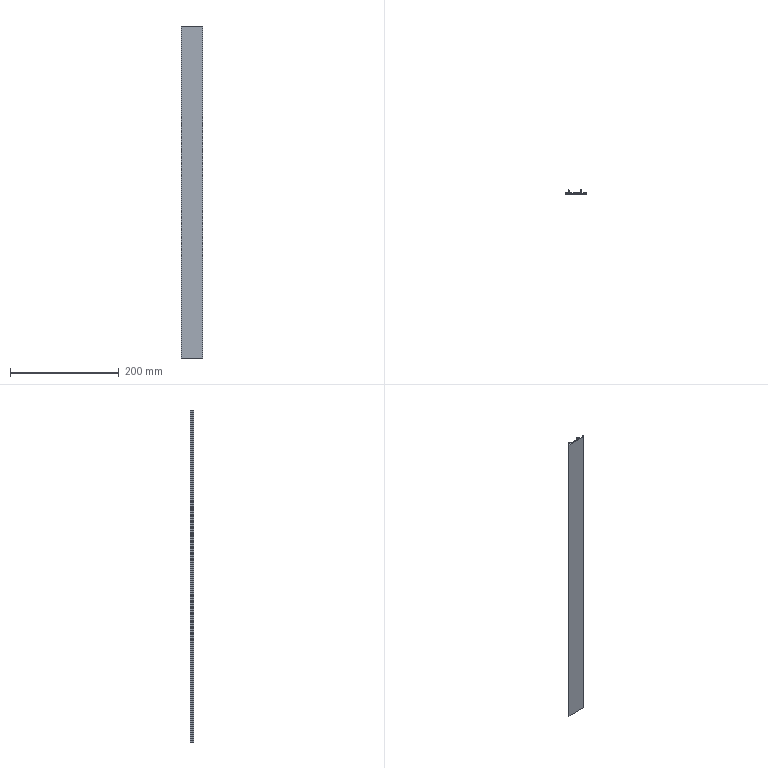Part | STEP file | STEP model-SOC30-610.step.STEP-427.STEP | 1 solid | 29 faces | box 40.225 x 7.254 x 610 mm | volume 58769 mm3 | cylinder 15 | plane 14 | commonest cylinder face diameters 2.54 x4 0.508 x3 1.524 x3 1.905 x3 6 x2
STEP:
#1=CARTESIAN_POINT('',(-35.814,-0.127,304.8));
#2=VERTEX_POINT('',#1);
#3=CARTESIAN_POINT('',(-35.052,-0.889,304.8));
#4=VERTEX_POINT('',#3);
#5=CARTESIAN_POINT('',(-35.052,-0.127,304.8));
#6=DIRECTION('',(0.,0.,1.));
#7=DIRECTION('',(1.,0.,0.));
#8=AXIS2_PLACEMENT_3D('',#5,#6,#7);
#9=CIRCLE('',#8,0.762);
#10=EDGE_CURVE('',#2,#4,#9,.T.);
#11=ORIENTED_EDGE('',*,*,#10,.T.);
#12=CARTESIAN_POINT('',(3.649,-0.889,304.8));
#13=VERTEX_POINT('',#12);
#14=CARTESIAN_POINT('',(-35.052,-0.889,304.8));
#15=DIRECTION('',(1.,0.,0.));
#16=VECTOR('',#15,1000.);
#17=LINE('',#14,#16);
#18=EDGE_CURVE('',#4,#13,#17,.T.);
#19=ORIENTED_EDGE('',*,*,#18,.T.);
#20=CARTESIAN_POINT('',(4.411,-0.127,304.8));
#21=VERTEX_POINT('',#20);
#22=CARTESIAN_POINT('',(3.649,-0.127,304.8));
#23=DIRECTION('',(0.,0.,1.));
#24=DIRECTION('',(1.,0.,0.));
#25=AXIS2_PLACEMENT_3D('',#22,#23,#24);
#26=CIRCLE('',#25,0.762);
#27=EDGE_CURVE('',#13,#21,#26,.T.);
#28=ORIENTED_EDGE('',*,*,#27,.T.);
#29=CARTESIAN_POINT('',(4.411,0.762,304.8));
#30=VERTEX_POINT('',#29);
#31=CARTESIAN_POINT('',(4.411,-0.127,304.8));
#32=DIRECTION('',(0.,1.,0.));
#33=VECTOR('',#32,1000.);
#34=LINE('',#31,#33);
#35=EDGE_CURVE('',#21,#30,#34,.T.);
#36=ORIENTED_EDGE('',*,*,#35,.T.);
#37=CARTESIAN_POINT('',(3.649,1.524,304.8));
#38=VERTEX_POINT('',#37);
#39=CARTESIAN_POINT('',(3.649,0.762,304.8));
#40=DIRECTION('',(0.,0.,1.));
#41=DIRECTION('',(1.,0.,0.));
#42=AXIS2_PLACEMENT_3D('',#39,#40,#41);
#43=CIRCLE('',#42,0.762);
#44=EDGE_CURVE('',#30,#38,#43,.T.);
#45=ORIENTED_EDGE('',*,*,#44,.T.);
#46=CARTESIAN_POINT('',(2.757,1.524,304.8));
#47=VERTEX_POINT('',#46);
#48=CARTESIAN_POINT('',(3.649,1.524,304.8));
#49=DIRECTION('',(-1.,0.,0.));
#50=VECTOR('',#49,1000.);
#51=LINE('',#48,#50);
#52=EDGE_CURVE('',#38,#47,#51,.T.);
#53=ORIENTED_EDGE('',*,*,#52,.T.);
#54=CARTESIAN_POINT('',(2.611,1.478,304.8));
#55=VERTEX_POINT('',#54);
#56=CARTESIAN_POINT('',(2.757,1.27,304.8));
#57=DIRECTION('',(0.,0.,1.));
#58=DIRECTION('',(1.,0.,0.));
#59=AXIS2_PLACEMENT_3D('',#56,#57,#58);
#60=CIRCLE('',#59,0.254);
#61=EDGE_CURVE('',#47,#55,#60,.T.);
#62=ORIENTED_EDGE('',*,*,#61,.T.);
#63=CARTESIAN_POINT('',(2.017,1.062,304.8));
#64=VERTEX_POINT('',#63);
#65=CARTESIAN_POINT('',(2.611,1.478,304.8));
#66=DIRECTION('',(-0.8192,-0.5736,0.));
#67=VECTOR('',#66,1000.);
#68=LINE('',#65,#67);
#69=EDGE_CURVE('',#55,#64,#68,.T.);
#70=ORIENTED_EDGE('',*,*,#69,.T.);
#71=CARTESIAN_POINT('',(1.871,1.016,304.8));
#72=VERTEX_POINT('',#71);
#73=CARTESIAN_POINT('',(1.871,1.27,304.8));
#74=DIRECTION('',(0.,0.,-1.));
#75=DIRECTION('',(-1.,0.,0.));
#76=AXIS2_PLACEMENT_3D('',#73,#74,#75);
#77=CIRCLE('',#76,0.254);
#78=EDGE_CURVE('',#64,#72,#77,.T.);
#79=ORIENTED_EDGE('',*,*,#78,.T.);
#80=CARTESIAN_POINT('',(-4.764,1.016,304.8));
#81=VERTEX_POINT('',#80);
#82=CARTESIAN_POINT('',(1.871,1.016,304.8));
#83=DIRECTION('',(-1.,0.,0.));
#84=VECTOR('',#83,1000.);
#85=LINE('',#82,#84);
#86=EDGE_CURVE('',#72,#81,#85,.T.);
#87=ORIENTED_EDGE('',*,*,#86,.T.);
#88=CARTESIAN_POINT('',(-6.034,2.286,304.8));
#89=VERTEX_POINT('',#88);
#90=CARTESIAN_POINT('',(-4.764,2.286,304.8));
#91=DIRECTION('',(0.,0.,-1.));
#92=DIRECTION('',(-1.,0.,0.));
#93=AXIS2_PLACEMENT_3D('',#90,#91,#92);
#94=CIRCLE('',#93,1.27);
#95=EDGE_CURVE('',#81,#89,#94,.T.);
#96=ORIENTED_EDGE('',*,*,#95,.T.);
#97=CARTESIAN_POINT('',(-6.034,4.016,304.8));
#98=VERTEX_POINT('',#97);
#99=CARTESIAN_POINT('',(-6.034,2.286,304.8));
#100=DIRECTION('',(0.,1.,0.));
#101=VECTOR('',#100,1000.);
#102=LINE('',#99,#101);
#103=EDGE_CURVE('',#89,#98,#102,.T.);
#104=ORIENTED_EDGE('',*,*,#103,.T.);
#105=CARTESIAN_POINT('',(-5.841,5.076,304.8));
#106=VERTEX_POINT('',#105);
#107=CARTESIAN_POINT('',(-3.034,4.016,304.8));
#108=DIRECTION('',(0.,0.,-1.));
#109=DIRECTION('',(-1.,0.,0.));
#110=AXIS2_PLACEMENT_3D('',#107,#108,#109);
#111=CIRCLE('',#110,3.);
#112=EDGE_CURVE('',#98,#106,#111,.T.);
#113=ORIENTED_EDGE('',*,*,#112,.T.);
#114=CARTESIAN_POINT('',(-5.779,5.412,304.8));
#115=VERTEX_POINT('',#114);
#116=CARTESIAN_POINT('',(-6.732,5.412,304.8));
#117=DIRECTION('',(0.,0.,1.));
#118=DIRECTION('',(1.,0.,0.));
#119=AXIS2_PLACEMENT_3D('',#116,#117,#118);
#120=CIRCLE('',#119,0.9525);
#121=EDGE_CURVE('',#106,#115,#120,.T.);
#122=ORIENTED_EDGE('',*,*,#121,.T.);
#123=CARTESIAN_POINT('',(-7.684,5.412,304.8));
#124=VERTEX_POINT('',#123);
#125=CARTESIAN_POINT('',(-6.732,5.412,304.8));
#126=DIRECTION('',(0.,0.,1.));
#127=DIRECTION('',(1.,0.,0.));
#128=AXIS2_PLACEMENT_3D('',#125,#126,#127);
#129=CIRCLE('',#128,0.9525);
#130=EDGE_CURVE('',#115,#124,#129,.T.);
#131=ORIENTED_EDGE('',*,*,#130,.T.);
#132=CARTESIAN_POINT('',(-7.684,2.286,304.8));
#133=VERTEX_POINT('',#132);
#134=CARTESIAN_POINT('',(-7.684,5.412,304.8));
#135=DIRECTION('',(0.,-1.,0.));
#136=VECTOR('',#135,1000.);
#137=LINE('',#134,#136);
#138=EDGE_CURVE('',#124,#133,#137,.T.);
#139=ORIENTED_EDGE('',*,*,#138,.T.);
#140=CARTESIAN_POINT('',(-8.954,1.016,304.8));
#141=VERTEX_POINT('',#140);
#142=CARTESIAN_POINT('',(-8.954,2.286,304.8));
#143=DIRECTION('',(0.,0.,-1.));
#144=DIRECTION('',(-1.,0.,0.));
#145=AXIS2_PLACEMENT_3D('',#142,#143,#144);
#146=CIRCLE('',#145,1.27);
#147=EDGE_CURVE('',#133,#141,#146,.T.);
#148=ORIENTED_EDGE('',*,*,#147,.T.);
#149=CARTESIAN_POINT('',(-27.114,1.016,304.8));
#150=VERTEX_POINT('',#149);
#151=CARTESIAN_POINT('',(-8.954,1.016,304.8));
#152=DIRECTION('',(-1.,0.,0.));
#153=VECTOR('',#152,1000.);
#154=LINE('',#151,#153);
#155=EDGE_CURVE('',#141,#150,#154,.T.);
#156=ORIENTED_EDGE('',*,*,#155,.T.);
#157=CARTESIAN_POINT('',(-28.384,2.286,304.8));
#158=VERTEX_POINT('',#157);
#159=CARTESIAN_POINT('',(-27.114,2.286,304.8));
#160=DIRECTION('',(0.,0.,-1.));
#161=DIRECTION('',(-1.,0.,0.));
#162=AXIS2_PLACEMENT_3D('',#159,#160,#161);
#163=CIRCLE('',#162,1.27);
#164=EDGE_CURVE('',#150,#158,#163,.T.);
#165=ORIENTED_EDGE('',*,*,#164,.T.);
#166=CARTESIAN_POINT('',(-28.384,5.412,304.8));
#167=VERTEX_POINT('',#166);
#168=CARTESIAN_POINT('',(-28.384,2.286,304.8));
#169=DIRECTION('',(0.,1.,0.));
#170=VECTOR('',#169,1000.);
#171=LINE('',#168,#170);
#172=EDGE_CURVE('',#158,#167,#171,.T.);
#173=ORIENTED_EDGE('',*,*,#172,.T.);
#174=CARTESIAN_POINT('',(-30.227,5.076,304.8));
#175=VERTEX_POINT('',#174);
#176=CARTESIAN_POINT('',(-29.336,5.412,304.8));
#177=DIRECTION('',(0.,0.,1.));
#178=DIRECTION('',(1.,0.,0.));
#179=AXIS2_PLACEMENT_3D('',#176,#177,#178);
#180=CIRCLE('',#179,0.9525);
#181=EDGE_CURVE('',#167,#175,#180,.T.);
#182=ORIENTED_EDGE('',*,*,#181,.T.);
#183=CARTESIAN_POINT('',(-30.034,4.016,304.8));
#184=VERTEX_POINT('',#183);
#185=CARTESIAN_POINT('',(-33.034,4.016,304.8));
#186=DIRECTION('',(0.,0.,-1.));
#187=DIRECTION('',(-1.,0.,0.));
#188=AXIS2_PLACEMENT_3D('',#185,#186,#187);
#189=CIRCLE('',#188,3.);
#190=EDGE_CURVE('',#175,#184,#189,.T.);
#191=ORIENTED_EDGE('',*,*,#190,.T.);
#192=CARTESIAN_POINT('',(-30.034,2.286,304.8));
#193=VERTEX_POINT('',#192);
#194=CARTESIAN_POINT('',(-30.034,4.016,304.8));
#195=DIRECTION('',(0.,-1.,0.));
#196=VECTOR('',#195,1000.);
#197=LINE('',#194,#196);
#198=EDGE_CURVE('',#184,#193,#197,.T.);
#199=ORIENTED_EDGE('',*,*,#198,.T.);
#200=CARTESIAN_POINT('',(-31.304,1.016,304.8));
#201=VERTEX_POINT('',#200);
#202=CARTESIAN_POINT('',(-31.304,2.286,304.8));
#203=DIRECTION('',(0.,0.,-1.));
#204=DIRECTION('',(-1.,0.,0.));
#205=AXIS2_PLACEMENT_3D('',#202,#203,#204);
#206=CIRCLE('',#205,1.27);
#207=EDGE_CURVE('',#193,#201,#206,.T.);
#208=ORIENTED_EDGE('',*,*,#207,.T.);
#209=CARTESIAN_POINT('',(-35.56,1.016,304.8));
#210=VERTEX_POINT('',#209);
#211=CARTESIAN_POINT('',(-31.304,1.016,304.8));
#212=DIRECTION('',(-1.,0.,0.));
#213=VECTOR('',#212,1000.);
#214=LINE('',#211,#213);
#215=EDGE_CURVE('',#201,#210,#214,.T.);
#216=ORIENTED_EDGE('',*,*,#215,.T.);
#217=CARTESIAN_POINT('',(-35.814,0.762,304.8));
#218=VERTEX_POINT('',#217);
#219=CARTESIAN_POINT('',(-35.56,0.762,304.8));
#220=DIRECTION('',(0.,0.,1.));
#221=DIRECTION('',(1.,0.,0.));
#222=AXIS2_PLACEMENT_3D('',#219,#220,#221);
#223=CIRCLE('',#222,0.254);
#224=EDGE_CURVE('',#210,#218,#223,.T.);
#225=ORIENTED_EDGE('',*,*,#224,.T.);
#226=CARTESIAN_POINT('',(-35.814,0.762,304.8));
#227=DIRECTION('',(0.,-1.,0.));
#228=VECTOR('',#227,1000.);
#229=LINE('',#226,#228);
#230=EDGE_CURVE('',#218,#2,#229,.T.);
#231=ORIENTED_EDGE('',*,*,#230,.T.);
#232=EDGE_LOOP('',(#11,#19,#28,#36,#45,#53,#62,#70,#79,#87,#96,#104,#113,#122,#131,#139,#148,#156,#165,#173,#182,#191,#199,#208,#216,#225,#231));
#233=FACE_OUTER_BOUND('',#232,.T.);
#234=CARTESIAN_POINT('',(-35.052,-0.127,304.8));
#235=DIRECTION('',(0.,0.,1.));
#236=DIRECTION('',(1.,0.,0.));
#237=AXIS2_PLACEMENT_3D('',#234,#235,#236);
#238=PLANE('',#237);
#239=ADVANCED_FACE('',(#233),#238,.T.);
#240=CARTESIAN_POINT('',(-35.814,-0.127,-305.2));
#241=VERTEX_POINT('',#240);
#242=CARTESIAN_POINT('',(-35.052,-0.889,-305.2));
#243=VERTEX_POINT('',#242);
#244=CARTESIAN_POINT('',(-35.052,-0.127,-305.2));
#245=DIRECTION('',(0.,0.,1.));
#246=DIRECTION('',(1.,0.,0.));
#247=AXIS2_PLACEMENT_3D('',#244,#245,#246);
#248=CIRCLE('',#247,0.762);
#249=EDGE_CURVE('',#241,#243,#248,.T.);
#250=ORIENTED_EDGE('',*,*,#249,.F.);
#251=CARTESIAN_POINT('',(-35.814,0.762,-305.2));
#252=VERTEX_POINT('',#251);
#253=CARTESIAN_POINT('',(-35.814,0.762,-305.2));
#254=DIRECTION('',(0.,-1.,0.));
#255=VECTOR('',#254,1000.);
#256=LINE('',#253,#255);
#257=EDGE_CURVE('',#252,#241,#256,.T.);
#258=ORIENTED_EDGE('',*,*,#257,.F.);
#259=CARTESIAN_POINT('',(-35.56,1.016,-305.2));
#260=VERTEX_POINT('',#259);
#261=CARTESIAN_POINT('',(-35.56,0.762,-305.2));
#262=DIRECTION('',(0.,0.,1.));
#263=DIRECTION('',(1.,0.,0.));
#264=AXIS2_PLACEMENT_3D('',#261,#262,#263);
#265=CIRCLE('',#264,0.254);
#266=EDGE_CURVE('',#260,#252,#265,.T.);
#267=ORIENTED_EDGE('',*,*,#266,.F.);
#268=CARTESIAN_POINT('',(-31.304,1.016,-305.2));
#269=VERTEX_POINT('',#268);
#270=CARTESIAN_POINT('',(-31.304,1.016,-305.2));
#271=DIRECTION('',(-1.,0.,0.));
#272=VECTOR('',#271,1000.);
#273=LINE('',#270,#272);
#274=EDGE_CURVE('',#269,#260,#273,.T.);
#275=ORIENTED_EDGE('',*,*,#274,.F.);
#276=CARTESIAN_POINT('',(-30.034,2.286,-305.2));
#277=VERTEX_POINT('',#276);
#278=CARTESIAN_POINT('',(-31.304,2.286,-305.2));
#279=DIRECTION('',(0.,0.,-1.));
#280=DIRECTION('',(-1.,0.,0.));
#281=AXIS2_PLACEMENT_3D('',#278,#279,#280);
#282=CIRCLE('',#281,1.27);
#283=EDGE_CURVE('',#277,#269,#282,.T.);
#284=ORIENTED_EDGE('',*,*,#283,.F.);
#285=CARTESIAN_POINT('',(-30.034,4.016,-305.2));
#286=VERTEX_POINT('',#285);
#287=CARTESIAN_POINT('',(-30.034,4.016,-305.2));
#288=DIRECTION('',(0.,-1.,0.));
#289=VECTOR('',#288,1000.);
#290=LINE('',#287,#289);
#291=EDGE_CURVE('',#286,#277,#290,.T.);
#292=ORIENTED_EDGE('',*,*,#291,.F.);
#293=CARTESIAN_POINT('',(-30.227,5.076,-305.2));
#294=VERTEX_POINT('',#293);
#295=CARTESIAN_POINT('',(-33.034,4.016,-305.2));
#296=DIRECTION('',(0.,0.,-1.));
#297=DIRECTION('',(-1.,0.,0.));
#298=AXIS2_PLACEMENT_3D('',#295,#296,#297);
#299=CIRCLE('',#298,3.);
#300=EDGE_CURVE('',#294,#286,#299,.T.);
#301=ORIENTED_EDGE('',*,*,#300,.F.);
#302=CARTESIAN_POINT('',(-28.384,5.412,-305.2));
#303=VERTEX_POINT('',#302);
#304=CARTESIAN_POINT('',(-29.336,5.412,-305.2));
#305=DIRECTION('',(0.,0.,1.));
#306=DIRECTION('',(1.,0.,0.));
#307=AXIS2_PLACEMENT_3D('',#304,#305,#306);
#308=CIRCLE('',#307,0.9525);
#309=EDGE_CURVE('',#303,#294,#308,.T.);
#310=ORIENTED_EDGE('',*,*,#309,.F.);
#311=CARTESIAN_POINT('',(-28.384,2.286,-305.2));
#312=VERTEX_POINT('',#311);
#313=CARTESIAN_POINT('',(-28.384,2.286,-305.2));
#314=DIRECTION('',(0.,1.,0.));
#315=VECTOR('',#314,1000.);
#316=LINE('',#313,#315);
#317=EDGE_CURVE('',#312,#303,#316,.T.);
#318=ORIENTED_EDGE('',*,*,#317,.F.);
#319=CARTESIAN_POINT('',(-27.114,1.016,-305.2));
#320=VERTEX_POINT('',#319);
#321=CARTESIAN_POINT('',(-27.114,2.286,-305.2));
#322=DIRECTION('',(0.,0.,-1.));
#323=DIRECTION('',(-1.,0.,0.));
#324=AXIS2_PLACEMENT_3D('',#321,#322,#323);
#325=CIRCLE('',#324,1.27);
#326=EDGE_CURVE('',#320,#312,#325,.T.);
#327=ORIENTED_EDGE('',*,*,#326,.F.);
#328=CARTESIAN_POINT('',(-8.954,1.016,-305.2));
#329=VERTEX_POINT('',#328);
#330=CARTESIAN_POINT('',(-8.954,1.016,-305.2));
#331=DIRECTION('',(-1.,0.,0.));
#332=VECTOR('',#331,1000.);
#333=LINE('',#330,#332);
#334=EDGE_CURVE('',#329,#320,#333,.T.);
#335=ORIENTED_EDGE('',*,*,#334,.F.);
#336=CARTESIAN_POINT('',(-7.684,2.286,-305.2));
#337=VERTEX_POINT('',#336);
#338=CARTESIAN_POINT('',(-8.954,2.286,-305.2));
#339=DIRECTION('',(0.,0.,-1.));
#340=DIRECTION('',(-1.,0.,0.));
#341=AXIS2_PLACEMENT_3D('',#338,#339,#340);
#342=CIRCLE('',#341,1.27);
#343=EDGE_CURVE('',#337,#329,#342,.T.);
#344=ORIENTED_EDGE('',*,*,#343,.F.);
#345=CARTESIAN_POINT('',(-7.684,5.412,-305.2));
#346=VERTEX_POINT('',#345);
#347=CARTESIAN_POINT('',(-7.684,5.412,-305.2));
#348=DIRECTION('',(0.,-1.,0.));
#349=VECTOR('',#348,1000.);
#350=LINE('',#347,#349);
#351=EDGE_CURVE('',#346,#337,#350,.T.);
#352=ORIENTED_EDGE('',*,*,#351,.F.);
#353=CARTESIAN_POINT('',(-5.779,5.412,-305.2));
#354=VERTEX_POINT('',#353);
#355=CARTESIAN_POINT('',(-6.732,5.412,-305.2));
#356=DIRECTION('',(0.,0.,1.));
#357=DIRECTION('',(1.,0.,0.));
#358=AXIS2_PLACEMENT_3D('',#355,#356,#357);
#359=CIRCLE('',#358,0.9525);
#360=EDGE_CURVE('',#354,#346,#359,.T.);
#361=ORIENTED_EDGE('',*,*,#360,.F.);
#362=CARTESIAN_POINT('',(-5.841,5.076,-305.2));
#363=VERTEX_POINT('',#362);
#364=CARTESIAN_POINT('',(-6.732,5.412,-305.2));
#365=DIRECTION('',(0.,0.,1.));
#366=DIRECTION('',(1.,0.,0.));
#367=AXIS2_PLACEMENT_3D('',#364,#365,#366);
#368=CIRCLE('',#367,0.9525);
#369=EDGE_CURVE('',#363,#354,#368,.T.);
#370=ORIENTED_EDGE('',*,*,#369,.F.);
#371=CARTESIAN_POINT('',(-6.034,4.016,-305.2));
#372=VERTEX_POINT('',#371);
#373=CARTESIAN_POINT('',(-3.034,4.016,-305.2));
#374=DIRECTION('',(0.,0.,-1.));
#375=DIRECTION('',(-1.,0.,0.));
#376=AXIS2_PLACEMENT_3D('',#373,#374,#375);
#377=CIRCLE('',#376,3.);
#378=EDGE_CURVE('',#372,#363,#377,.T.);
#379=ORIENTED_EDGE('',*,*,#378,.F.);
#380=CARTESIAN_POINT('',(-6.034,2.286,-305.2));
#381=VERTEX_POINT('',#380);
#382=CARTESIAN_POINT('',(-6.034,2.286,-305.2));
#383=DIRECTION('',(0.,1.,0.));
#384=VECTOR('',#383,1000.);
#385=LINE('',#382,#384);
#386=EDGE_CURVE('',#381,#372,#385,.T.);
#387=ORIENTED_EDGE('',*,*,#386,.F.);
#388=CARTESIAN_POINT('',(-4.764,1.016,-305.2));
#389=VERTEX_POINT('',#388);
#390=CARTESIAN_POINT('',(-4.764,2.286,-305.2));
#391=DIRECTION('',(0.,0.,-1.));
#392=DIRECTION('',(-1.,0.,0.));
#393=AXIS2_PLACEMENT_3D('',#390,#391,#392);
#394=CIRCLE('',#393,1.27);
#395=EDGE_CURVE('',#389,#381,#394,.T.);
#396=ORIENTED_EDGE('',*,*,#395,.F.);
#397=CARTESIAN_POINT('',(1.871,1.016,-305.2));
#398=VERTEX_POINT('',#397);
#399=CARTESIAN_POINT('',(1.871,1.016,-305.2));
#400=DIRECTION('',(-1.,0.,0.));
#401=VECTOR('',#400,1000.);
#402=LINE('',#399,#401);
#403=EDGE_CURVE('',#398,#389,#402,.T.);
#404=ORIENTED_EDGE('',*,*,#403,.F.);
#405=CARTESIAN_POINT('',(2.017,1.062,-305.2));
#406=VERTEX_POINT('',#405);
#407=CARTESIAN_POINT('',(1.871,1.27,-305.2));
#408=DIRECTION('',(0.,0.,-1.));
#409=DIRECTION('',(-1.,0.,0.));
#410=AXIS2_PLACEMENT_3D('',#407,#408,#409);
#411=CIRCLE('',#410,0.254);
#412=EDGE_CURVE('',#406,#398,#411,.T.);
#413=ORIENTED_EDGE('',*,*,#412,.F.);
#414=CARTESIAN_POINT('',(2.611,1.478,-305.2));
#415=VERTEX_POINT('',#414);
#416=CARTESIAN_POINT('',(2.611,1.478,-305.2));
#417=DIRECTION('',(-0.8192,-0.5736,0.));
#418=VECTOR('',#417,1000.);
#419=LINE('',#416,#418);
#420=EDGE_CURVE('',#415,#406,#419,.T.);
#421=ORIENTED_EDGE('',*,*,#420,.F.);
#422=CARTESIAN_POINT('',(2.757,1.524,-305.2));
#423=VERTEX_POINT('',#422);
#424=CARTESIAN_POINT('',(2.757,1.27,-305.2));
#425=DIRECTION('',(0.,0.,1.));
#426=DIRECTION('',(1.,0.,0.));
#427=AXIS2_PLACEMENT_3D('',#424,#425,#426);
#428=CIRCLE('',#427,0.254);
#429=EDGE_CURVE('',#423,#415,#428,.T.);
#430=ORIENTED_EDGE('',*,*,#429,.F.);
#431=CARTESIAN_POINT('',(3.649,1.524,-305.2));
#432=VERTEX_POINT('',#431);
#433=CARTESIAN_POINT('',(3.649,1.524,-305.2));
#434=DIRECTION('',(-1.,0.,0.));
#435=VECTOR('',#434,1000.);
#436=LINE('',#433,#435);
#437=EDGE_CURVE('',#432,#423,#436,.T.);
#438=ORIENTED_EDGE('',*,*,#437,.F.);
#439=CARTESIAN_POINT('',(4.411,0.762,-305.2));
#440=VERTEX_POINT('',#439);
#441=CARTESIAN_POINT('',(3.649,0.762,-305.2));
#442=DIRECTION('',(0.,0.,1.));
#443=DIRECTION('',(1.,0.,0.));
#444=AXIS2_PLACEMENT_3D('',#441,#442,#443);
#445=CIRCLE('',#444,0.762);
#446=EDGE_CURVE('',#440,#432,#445,.T.);
#447=ORIENTED_EDGE('',*,*,#446,.F.);
#448=CARTESIAN_POINT('',(4.411,-0.127,-305.2));
#449=VERTEX_POINT('',#448);
#450=CARTESIAN_POINT('',(4.411,-0.127,-305.2));
#451=DIRECTION('',(0.,1.,0.));
#452=VECTOR('',#451,1000.);
#453=LINE('',#450,#452);
#454=EDGE_CURVE('',#449,#440,#453,.T.);
#455=ORIENTED_EDGE('',*,*,#454,.F.);
#456=CARTESIAN_POINT('',(3.649,-0.889,-305.2));
#457=VERTEX_POINT('',#456);
#458=CARTESIAN_POINT('',(3.649,-0.127,-305.2));
#459=DIRECTION('',(0.,0.,1.));
#460=DIRECTION('',(1.,0.,0.));
#461=AXIS2_PLACEMENT_3D('',#458,#459,#460);
#462=CIRCLE('',#461,0.762);
#463=EDGE_CURVE('',#457,#449,#462,.T.);
#464=ORIENTED_EDGE('',*,*,#463,.F.);
#465=CARTESIAN_POINT('',(-35.052,-0.889,-305.2));
#466=DIRECTION('',(1.,0.,0.));
#467=VECTOR('',#466,1000.);
#468=LINE('',#465,#467);
#469=EDGE_CURVE('',#243,#457,#468,.T.);
#470=ORIENTED_EDGE('',*,*,#469,.F.);
#471=EDGE_LOOP('',(#250,#258,#267,#275,#284,#292,#301,#310,#318,#327,#335,#344,#352,#361,#370,#379,#387,#396,#404,#413,#421,#430,#438,#447,#455,#464,#470));
#472=FACE_OUTER_BOUND('',#471,.T.);
#473=CARTESIAN_POINT('',(-35.052,-0.127,-305.2));
#474=DIRECTION('',(0.,0.,1.));
#475=DIRECTION('',(1.,0.,0.));
#476=AXIS2_PLACEMENT_3D('',#473,#474,#475);
#477=PLANE('',#476);
#478=ADVANCED_FACE('',(#472),#477,.F.);
#479=ORIENTED_EDGE('',*,*,#18,.F.);
#480=CARTESIAN_POINT('',(-35.052,-0.889,-305.2));
#481=DIRECTION('',(0.,0.,1.));
#482=VECTOR('',#481,1000.);
#483=LINE('',#480,#482);
#484=EDGE_CURVE('',#243,#4,#483,.T.);
#485=ORIENTED_EDGE('',*,*,#484,.F.);
#486=ORIENTED_EDGE('',*,*,#469,.T.);
#487=CARTESIAN_POINT('',(3.649,-0.889,-305.2));
#488=DIRECTION('',(0.,0.,1.));
#489=VECTOR('',#488,1000.);
#490=LINE('',#487,#489);
#491=EDGE_CURVE('',#457,#13,#490,.T.);
#492=ORIENTED_EDGE('',*,*,#491,.T.);
#493=EDGE_LOOP('',(#479,#485,#486,#492));
#494=FACE_OUTER_BOUND('',#493,.T.);
#495=CARTESIAN_POINT('',(-35.052,-0.889,-305.2));
#496=DIRECTION('',(0.,-1.,0.));
#497=DIRECTION('',(0.,0.,-1.));
#498=AXIS2_PLACEMENT_3D('',#495,#496,#497);
#499=PLANE('',#498);
#500=ADVANCED_FACE('',(#494),#499,.T.);
#501=ORIENTED_EDGE('',*,*,#27,.F.);
#502=ORIENTED_EDGE('',*,*,#491,.F.);
#503=ORIENTED_EDGE('',*,*,#463,.T.);
#504=CARTESIAN_POINT('',(4.411,-0.127,-305.2));
#505=DIRECTION('',(0.,0.,1.));
#506=VECTOR('',#505,1000.);
#507=LINE('',#504,#506);
#508=EDGE_CURVE('',#449,#21,#507,.T.);
#509=ORIENTED_EDGE('',*,*,#508,.T.);
#510=EDGE_LOOP('',(#501,#502,#503,#509));
#511=FACE_OUTER_BOUND('',#510,.T.);
#512=CARTESIAN_POINT('',(3.649,-0.127,-305.2));
#513=DIRECTION('',(0.,0.,1.));
#514=DIRECTION('',(1.,0.,0.));
#515=AXIS2_PLACEMENT_3D('',#512,#513,#514);
#516=CYLINDRICAL_SURFACE('',#515,0.762);
#517=ADVANCED_FACE('',(#511),#516,.T.);
#518=ORIENTED_EDGE('',*,*,#35,.F.);
#519=ORIENTED_EDGE('',*,*,#508,.F.);
#520=ORIENTED_EDGE('',*,*,#454,.T.);
#521=CARTESIAN_POINT('',(4.411,0.762,-305.2));
#522=DIRECTION('',(0.,0.,1.));
#523=VECTOR('',#522,1000.);
#524=LINE('',#521,#523);
#525=EDGE_CURVE('',#440,#30,#524,.T.);
#526=ORIENTED_EDGE('',*,*,#525,.T.);
#527=EDGE_LOOP('',(#518,#519,#520,#526));
#528=FACE_OUTER_BOUND('',#527,.T.);
#529=CARTESIAN_POINT('',(4.411,-0.127,-305.2));
#530=DIRECTION('',(1.,0.,0.));
#531=DIRECTION('',(0.,-1.,0.));
#532=AXIS2_PLACEMENT_3D('',#529,#530,#531);
#533=PLANE('',#532);
#534=ADVANCED_FACE('',(#528),#533,.T.);
#535=ORIENTED_EDGE('',*,*,#44,.F.);
#536=ORIENTED_EDGE('',*,*,#525,.F.);
#537=ORIENTED_EDGE('',*,*,#446,.T.);
#538=CARTESIAN_POINT('',(3.649,1.524,-305.2));
#539=DIRECTION('',(0.,0.,1.));
#540=VECTOR('',#539,1000.);
#541=LINE('',#538,#540);
#542=EDGE_CURVE('',#432,#38,#541,.T.);
#543=ORIENTED_EDGE('',*,*,#542,.T.);
#544=EDGE_LOOP('',(#535,#536,#537,#543));
#545=FACE_OUTER_BOUND('',#544,.T.);
#546=CARTESIAN_POINT('',(3.649,0.762,-305.2));
#547=DIRECTION('',(0.,0.,1.));
#548=DIRECTION('',(1.,0.,0.));
#549=AXIS2_PLACEMENT_3D('',#546,#547,#548);
#550=CYLINDRICAL_SURFACE('',#549,0.762);
#551=ADVANCED_FACE('',(#545),#550,.T.);
#552=ORIENTED_EDGE('',*,*,#52,.F.);
#553=ORIENTED_EDGE('',*,*,#542,.F.);
#554=ORIENTED_EDGE('',*,*,#437,.T.);
#555=CARTESIAN_POINT('',(2.757,1.524,-305.2));
#556=DIRECTION('',(0.,0.,1.));
#557=VECTOR('',#556,1000.);
#558=LINE('',#555,#557);
#559=EDGE_CURVE('',#423,#47,#558,.T.);
#560=ORIENTED_EDGE('',*,*,#559,.T.);
#561=EDGE_LOOP('',(#552,#553,#554,#560));
#562=FACE_OUTER_BOUND('',#561,.T.);
#563=CARTESIAN_POINT('',(3.649,1.524,-305.2));
#564=DIRECTION('',(0.,1.,0.));
#565=DIRECTION('',(1.,0.,0.));
#566=AXIS2_PLACEMENT_3D('',#563,#564,#565);
#567=PLANE('',#566);
#568=ADVANCED_FACE('',(#562),#567,.T.);
#569=ORIENTED_EDGE('',*,*,#61,.F.);
#570=ORIENTED_EDGE('',*,*,#559,.F.);
#571=ORIENTED_EDGE('',*,*,#429,.T.);
#572=CARTESIAN_POINT('',(2.611,1.478,-305.2));
#573=DIRECTION('',(0.,0.,1.));
#574=VECTOR('',#573,1000.);
#575=LINE('',#572,#574);
#576=EDGE_CURVE('',#415,#55,#575,.T.);
#577=ORIENTED_EDGE('',*,*,#576,.T.);
#578=EDGE_LOOP('',(#569,#570,#571,#577));
#579=FACE_OUTER_BOUND('',#578,.T.);
#580=CARTESIAN_POINT('',(2.757,1.27,-305.2));
#581=DIRECTION('',(0.,0.,1.));
#582=DIRECTION('',(1.,0.,0.));
#583=AXIS2_PLACEMENT_3D('',#580,#581,#582);
#584=CYLINDRICAL_SURFACE('',#583,0.254);
#585=ADVANCED_FACE('',(#579),#584,.T.);
#586=ORIENTED_EDGE('',*,*,#69,.F.);
#587=ORIENTED_EDGE('',*,*,#576,.F.);
#588=ORIENTED_EDGE('',*,*,#420,.T.);
#589=CARTESIAN_POINT('',(2.017,1.062,-305.2));
#590=DIRECTION('',(0.,0.,1.));
#591=VECTOR('',#590,1000.);
#592=LINE('',#589,#591);
#593=EDGE_CURVE('',#406,#64,#592,.T.);
#594=ORIENTED_EDGE('',*,*,#593,.T.);
#595=EDGE_LOOP('',(#586,#587,#588,#594));
#596=FACE_OUTER_BOUND('',#595,.T.);
#597=CARTESIAN_POINT('',(2.611,1.478,-305.2));
#598=DIRECTION('',(-0.5736,0.8192,0.));
#599=DIRECTION('',(0.,0.,1.));
#600=AXIS2_PLACEMENT_3D('',#597,#598,#599);
#601=PLANE('',#600);
#602=ADVANCED_FACE('',(#596),#601,.T.);
#603=ORIENTED_EDGE('',*,*,#78,.F.);
#604=ORIENTED_EDGE('',*,*,#593,.F.);
#605=ORIENTED_EDGE('',*,*,#412,.T.);
#606=CARTESIAN_POINT('',(1.871,1.016,-305.2));
#607=DIRECTION('',(0.,0.,1.));
#608=VECTOR('',#607,1000.);
#609=LINE('',#606,#608);
#610=EDGE_CURVE('',#398,#72,#609,.T.);
#611=ORIENTED_EDGE('',*,*,#610,.T.);
#612=EDGE_LOOP('',(#603,#604,#605,#611));
#613=FACE_OUTER_BOUND('',#612,.T.);
#614=CARTESIAN_POINT('',(1.871,1.27,-305.2));
#615=DIRECTION('',(0.,0.,1.));
#616=DIRECTION('',(1.,0.,0.));
#617=AXIS2_PLACEMENT_3D('',#614,#615,#616);
#618=CYLINDRICAL_SURFACE('',#617,0.254);
#619=ADVANCED_FACE('',(#613),#618,.F.);
#620=ORIENTED_EDGE('',*,*,#86,.F.);
#621=ORIENTED_EDGE('',*,*,#610,.F.);
#622=ORIENTED_EDGE('',*,*,#403,.T.);
#623=CARTESIAN_POINT('',(-4.764,1.016,-305.2));
#624=DIRECTION('',(0.,0.,1.));
#625=VECTOR('',#624,1000.);
#626=LINE('',#623,#625);
#627=EDGE_CURVE('',#389,#81,#626,.T.);
#628=ORIENTED_EDGE('',*,*,#627,.T.);
#629=EDGE_LOOP('',(#620,#621,#622,#628));
#630=FACE_OUTER_BOUND('',#629,.T.);
#631=CARTESIAN_POINT('',(1.871,1.016,-305.2));
#632=DIRECTION('',(0.,1.,0.));
#633=DIRECTION('',(1.,0.,0.));
#634=AXIS2_PLACEMENT_3D('',#631,#632,#633);
#635=PLANE('',#634);
#636=ADVANCED_FACE('',(#630),#635,.T.);
#637=ORIENTED_EDGE('',*,*,#95,.F.);
#638=ORIENTED_EDGE('',*,*,#627,.F.);
#639=ORIENTED_EDGE('',*,*,#395,.T.);
#640=CARTESIAN_POINT('',(-6.034,2.286,-305.2));
#641=DIRECTION('',(0.,0.,1.));
#642=VECTOR('',#641,1000.);
#643=LINE('',#640,#642);
#644=EDGE_CURVE('',#381,#89,#643,.T.);
#645=ORIENTED_EDGE('',*,*,#644,.T.);
#646=EDGE_LOOP('',(#637,#638,#639,#645));
#647=FACE_OUTER_BOUND('',#646,.T.);
#648=CARTESIAN_POINT('',(-4.764,2.286,-305.2));
#649=DIRECTION('',(0.,0.,1.));
#650=DIRECTION('',(1.,0.,0.));
#651=AXIS2_PLACEMENT_3D('',#648,#649,#650);
#652=CYLINDRICAL_SURFACE('',#651,1.27);
#653=ADVANCED_FACE('',(#647),#652,.F.);
#654=ORIENTED_EDGE('',*,*,#103,.F.);
#655=ORIENTED_EDGE('',*,*,#644,.F.);
#656=ORIENTED_EDGE('',*,*,#386,.T.);
#657=CARTESIAN_POINT('',(-6.034,4.016,-305.2));
#658=DIRECTION('',(0.,0.,1.));
#659=VECTOR('',#658,1000.);
#660=LINE('',#657,#659);
#661=EDGE_CURVE('',#372,#98,#660,.T.);
#662=ORIENTED_EDGE('',*,*,#661,.T.);
#663=EDGE_LOOP('',(#654,#655,#656,#662));
#664=FACE_OUTER_BOUND('',#663,.T.);
#665=CARTESIAN_POINT('',(-6.034,2.286,-305.2));
#666=DIRECTION('',(1.,0.,0.));
#667=DIRECTION('',(0.,1.,0.));
#668=AXIS2_PLACEMENT_3D('',#665,#666,#667);
#669=PLANE('',#668);
#670=ADVANCED_FACE('',(#664),#669,.T.);
#671=ORIENTED_EDGE('',*,*,#112,.F.);
#672=ORIENTED_EDGE('',*,*,#661,.F.);
#673=ORIENTED_EDGE('',*,*,#378,.T.);
#674=CARTESIAN_POINT('',(-5.841,5.076,-305.2));
#675=DIRECTION('',(0.,0.,1.));
#676=VECTOR('',#675,1000.);
#677=LINE('',#674,#676);
#678=EDGE_CURVE('',#363,#106,#677,.T.);
#679=ORIENTED_EDGE('',*,*,#678,.T.);
#680=EDGE_LOOP('',(#671,#672,#673,#679));
#681=FACE_OUTER_BOUND('',#680,.T.);
#682=CARTESIAN_POINT('',(-3.034,4.016,-305.2));
#683=DIRECTION('',(0.,0.,1.));
#684=DIRECTION('',(1.,0.,0.));
#685=AXIS2_PLACEMENT_3D('',#682,#683,#684);
#686=CYLINDRICAL_SURFACE('',#685,3.);
#687=ADVANCED_FACE('',(#681),#686,.F.);
#688=CARTESIAN_POINT('',(-5.779,5.412,-305.2));
#689=DIRECTION('',(0.,0.,1.));
#690=VECTOR('',#689,1000.);
#691=LINE('',#688,#690);
#692=EDGE_CURVE('',#354,#115,#691,.T.);
#693=ORIENTED_EDGE('',*,*,#692,.F.);
#694=ORIENTED_EDGE('',*,*,#360,.T.);
#695=CARTESIAN_POINT('',(-7.684,5.412,-305.2));
#696=DIRECTION('',(0.,0.,1.));
#697=VECTOR('',#696,1000.);
#698=LINE('',#695,#697);
#699=EDGE_CURVE('',#346,#124,#698,.T.);
#700=ORIENTED_EDGE('',*,*,#699,.T.);
#701=ORIENTED_EDGE('',*,*,#130,.F.);
#702=EDGE_LOOP('',(#693,#694,#700,#701));
#703=FACE_OUTER_BOUND('',#702,.T.);
#704=CARTESIAN_POINT('',(-6.732,5.412,-305.2));
#705=DIRECTION('',(0.,0.,1.));
#706=DIRECTION('',(1.,0.,0.));
#707=AXIS2_PLACEMENT_3D('',#704,#705,#706);
#708=CYLINDRICAL_SURFACE('',#707,0.9525);
#709=ADVANCED_FACE('',(#703),#708,.T.);
#710=ORIENTED_EDGE('',*,*,#138,.F.);
#711=ORIENTED_EDGE('',*,*,#699,.F.);
#712=ORIENTED_EDGE('',*,*,#351,.T.);
#713=CARTESIAN_POINT('',(-7.684,2.286,-305.2));
#714=DIRECTION('',(0.,0.,1.));
#715=VECTOR('',#714,1000.);
#716=LINE('',#713,#715);
#717=EDGE_CURVE('',#337,#133,#716,.T.);
#718=ORIENTED_EDGE('',*,*,#717,.T.);
#719=EDGE_LOOP('',(#710,#711,#712,#718));
#720=FACE_OUTER_BOUND('',#719,.T.);
#721=CARTESIAN_POINT('',(-7.684,5.412,-305.2));
#722=DIRECTION('',(-1.,0.,0.));
#723=DIRECTION('',(0.,0.,1.));
#724=AXIS2_PLACEMENT_3D('',#721,#722,#723);
#725=PLANE('',#724);
#726=ADVANCED_FACE('',(#720),#725,.T.);
#727=ORIENTED_EDGE('',*,*,#147,.F.);
#728=ORIENTED_EDGE('',*,*,#717,.F.);
#729=ORIENTED_EDGE('',*,*,#343,.T.);
#730=CARTESIAN_POINT('',(-8.954,1.016,-305.2));
#731=DIRECTION('',(0.,0.,1.));
#732=VECTOR('',#731,1000.);
#733=LINE('',#730,#732);
#734=EDGE_CURVE('',#329,#141,#733,.T.);
#735=ORIENTED_EDGE('',*,*,#734,.T.);
#736=EDGE_LOOP('',(#727,#728,#729,#735));
#737=FACE_OUTER_BOUND('',#736,.T.);
#738=CARTESIAN_POINT('',(-8.954,2.286,-305.2));
#739=DIRECTION('',(0.,0.,1.));
#740=DIRECTION('',(1.,0.,0.));
#741=AXIS2_PLACEMENT_3D('',#738,#739,#740);
#742=CYLINDRICAL_SURFACE('',#741,1.27);
#743=ADVANCED_FACE('',(#737),#742,.F.);
#744=ORIENTED_EDGE('',*,*,#155,.F.);
#745=ORIENTED_EDGE('',*,*,#734,.F.);
#746=ORIENTED_EDGE('',*,*,#334,.T.);
#747=CARTESIAN_POINT('',(-27.114,1.016,-305.2));
#748=DIRECTION('',(0.,0.,1.));
#749=VECTOR('',#748,1000.);
#750=LINE('',#747,#749);
#751=EDGE_CURVE('',#320,#150,#750,.T.);
#752=ORIENTED_EDGE('',*,*,#751,.T.);
#753=EDGE_LOOP('',(#744,#745,#746,#752));
#754=FACE_OUTER_BOUND('',#753,.T.);
#755=CARTESIAN_POINT('',(-8.954,1.016,-305.2));
#756=DIRECTION('',(0.,1.,0.));
#757=DIRECTION('',(1.,0.,0.));
#758=AXIS2_PLACEMENT_3D('',#755,#756,#757);
#759=PLANE('',#758);
#760=ADVANCED_FACE('',(#754),#759,.T.);
#761=ORIENTED_EDGE('',*,*,#164,.F.);
#762=ORIENTED_EDGE('',*,*,#751,.F.);
#763=ORIENTED_EDGE('',*,*,#326,.T.);
#764=CARTESIAN_POINT('',(-28.384,2.286,-305.2));
#765=DIRECTION('',(0.,0.,1.));
#766=VECTOR('',#765,1000.);
#767=LINE('',#764,#766);
#768=EDGE_CURVE('',#312,#158,#767,.T.);
#769=ORIENTED_EDGE('',*,*,#768,.T.);
#770=EDGE_LOOP('',(#761,#762,#763,#769));
#771=FACE_OUTER_BOUND('',#770,.T.);
#772=CARTESIAN_POINT('',(-27.114,2.286,-305.2));
#773=DIRECTION('',(0.,0.,1.));
#774=DIRECTION('',(1.,0.,0.));
#775=AXIS2_PLACEMENT_3D('',#772,#773,#774);
#776=CYLINDRICAL_SURFACE('',#775,1.27);
#777=ADVANCED_FACE('',(#771),#776,.F.);
#778=ORIENTED_EDGE('',*,*,#172,.F.);
#779=ORIENTED_EDGE('',*,*,#768,.F.);
#780=ORIENTED_EDGE('',*,*,#317,.T.);
#781=CARTESIAN_POINT('',(-28.384,5.412,-305.2));
#782=DIRECTION('',(0.,0.,1.));
#783=VECTOR('',#782,1000.);
#784=LINE('',#781,#783);
#785=EDGE_CURVE('',#303,#167,#784,.T.);
#786=ORIENTED_EDGE('',*,*,#785,.T.);
#787=EDGE_LOOP('',(#778,#779,#780,#786));
#788=FACE_OUTER_BOUND('',#787,.T.);
#789=CARTESIAN_POINT('',(-28.384,2.286,-305.2));
#790=DIRECTION('',(1.,0.,0.));
#791=DIRECTION('',(0.,-1.,0.));
#792=AXIS2_PLACEMENT_3D('',#789,#790,#791);
#793=PLANE('',#792);
#794=ADVANCED_FACE('',(#788),#793,.T.);
#795=ORIENTED_EDGE('',*,*,#181,.F.);
#796=ORIENTED_EDGE('',*,*,#785,.F.);
#797=ORIENTED_EDGE('',*,*,#309,.T.);
#798=CARTESIAN_POINT('',(-30.227,5.076,-305.2));
#799=DIRECTION('',(0.,0.,1.));
#800=VECTOR('',#799,1000.);
#801=LINE('',#798,#800);
#802=EDGE_CURVE('',#294,#175,#801,.T.);
#803=ORIENTED_EDGE('',*,*,#802,.T.);
#804=EDGE_LOOP('',(#795,#796,#797,#803));
#805=FACE_OUTER_BOUND('',#804,.T.);
#806=CARTESIAN_POINT('',(-29.336,5.412,-305.2));
#807=DIRECTION('',(0.,0.,1.));
#808=DIRECTION('',(1.,0.,0.));
#809=AXIS2_PLACEMENT_3D('',#806,#807,#808);
#810=CYLINDRICAL_SURFACE('',#809,0.9525);
#811=ADVANCED_FACE('',(#805),#810,.T.);
#812=ORIENTED_EDGE('',*,*,#190,.F.);
#813=ORIENTED_EDGE('',*,*,#802,.F.);
#814=ORIENTED_EDGE('',*,*,#300,.T.);
#815=CARTESIAN_POINT('',(-30.034,4.016,-305.2));
#816=DIRECTION('',(0.,0.,1.));
#817=VECTOR('',#816,1000.);
#818=LINE('',#815,#817);
#819=EDGE_CURVE('',#286,#184,#818,.T.);
#820=ORIENTED_EDGE('',*,*,#819,.T.);
#821=EDGE_LOOP('',(#812,#813,#814,#820));
#822=FACE_OUTER_BOUND('',#821,.T.);
#823=CARTESIAN_POINT('',(-33.034,4.016,-305.2));
#824=DIRECTION('',(0.,0.,1.));
#825=DIRECTION('',(1.,0.,0.));
#826=AXIS2_PLACEMENT_3D('',#823,#824,#825);
#827=CYLINDRICAL_SURFACE('',#826,3.);
#828=ADVANCED_FACE('',(#822),#827,.F.);
#829=ORIENTED_EDGE('',*,*,#198,.F.);
#830=ORIENTED_EDGE('',*,*,#819,.F.);
#831=ORIENTED_EDGE('',*,*,#291,.T.);
#832=CARTESIAN_POINT('',(-30.034,2.286,-305.2));
#833=DIRECTION('',(0.,0.,1.));
#834=VECTOR('',#833,1000.);
#835=LINE('',#832,#834);
#836=EDGE_CURVE('',#277,#193,#835,.T.);
#837=ORIENTED_EDGE('',*,*,#836,.T.);
#838=EDGE_LOOP('',(#829,#830,#831,#837));
#839=FACE_OUTER_BOUND('',#838,.T.);
#840=CARTESIAN_POINT('',(-30.034,4.016,-305.2));
#841=DIRECTION('',(-1.,0.,0.));
#842=DIRECTION('',(0.,0.,1.));
#843=AXIS2_PLACEMENT_3D('',#840,#841,#842);
#844=PLANE('',#843);
#845=ADVANCED_FACE('',(#839),#844,.T.);
#846=ORIENTED_EDGE('',*,*,#207,.F.);
#847=ORIENTED_EDGE('',*,*,#836,.F.);
#848=ORIENTED_EDGE('',*,*,#283,.T.);
#849=CARTESIAN_POINT('',(-31.304,1.016,-305.2));
#850=DIRECTION('',(0.,0.,1.));
#851=VECTOR('',#850,1000.);
#852=LINE('',#849,#851);
#853=EDGE_CURVE('',#269,#201,#852,.T.);
#854=ORIENTED_EDGE('',*,*,#853,.T.);
#855=EDGE_LOOP('',(#846,#847,#848,#854));
#856=FACE_OUTER_BOUND('',#855,.T.);
#857=CARTESIAN_POINT('',(-31.304,2.286,-305.2));
#858=DIRECTION('',(0.,0.,1.));
#859=DIRECTION('',(1.,0.,0.));
#860=AXIS2_PLACEMENT_3D('',#857,#858,#859);
#861=CYLINDRICAL_SURFACE('',#860,1.27);
#862=ADVANCED_FACE('',(#856),#861,.F.);
#863=ORIENTED_EDGE('',*,*,#215,.F.);
#864=ORIENTED_EDGE('',*,*,#853,.F.);
#865=ORIENTED_EDGE('',*,*,#274,.T.);
#866=CARTESIAN_POINT('',(-35.56,1.016,-305.2));
#867=DIRECTION('',(0.,0.,1.));
#868=VECTOR('',#867,1000.);
#869=LINE('',#866,#868);
#870=EDGE_CURVE('',#260,#210,#869,.T.);
#871=ORIENTED_EDGE('',*,*,#870,.T.);
#872=EDGE_LOOP('',(#863,#864,#865,#871));
#873=FACE_OUTER_BOUND('',#872,.T.);
#874=CARTESIAN_POINT('',(-31.304,1.016,-305.2));
#875=DIRECTION('',(0.,1.,0.));
#876=DIRECTION('',(1.,0.,0.));
#877=AXIS2_PLACEMENT_3D('',#874,#875,#876);
#878=PLANE('',#877);
#879=ADVANCED_FACE('',(#873),#878,.T.);
#880=ORIENTED_EDGE('',*,*,#224,.F.);
#881=ORIENTED_EDGE('',*,*,#870,.F.);
#882=ORIENTED_EDGE('',*,*,#266,.T.);
#883=CARTESIAN_POINT('',(-35.814,0.762,-305.2));
#884=DIRECTION('',(0.,0.,1.));
#885=VECTOR('',#884,1000.);
#886=LINE('',#883,#885);
#887=EDGE_CURVE('',#252,#218,#886,.T.);
#888=ORIENTED_EDGE('',*,*,#887,.T.);
#889=EDGE_LOOP('',(#880,#881,#882,#888));
#890=FACE_OUTER_BOUND('',#889,.T.);
#891=CARTESIAN_POINT('',(-35.56,0.762,-305.2));
#892=DIRECTION('',(0.,0.,1.));
#893=DIRECTION('',(1.,0.,0.));
#894=AXIS2_PLACEMENT_3D('',#891,#892,#893);
#895=CYLINDRICAL_SURFACE('',#894,0.254);
#896=ADVANCED_FACE('',(#890),#895,.T.);
#897=ORIENTED_EDGE('',*,*,#230,.F.);
#898=ORIENTED_EDGE('',*,*,#887,.F.);
#899=ORIENTED_EDGE('',*,*,#257,.T.);
#900=CARTESIAN_POINT('',(-35.814,-0.127,-305.2));
#901=DIRECTION('',(0.,0.,1.));
#902=VECTOR('',#901,1000.);
#903=LINE('',#900,#902);
#904=EDGE_CURVE('',#241,#2,#903,.T.);
#905=ORIENTED_EDGE('',*,*,#904,.T.);
#906=EDGE_LOOP('',(#897,#898,#899,#905));
#907=FACE_OUTER_BOUND('',#906,.T.);
#908=CARTESIAN_POINT('',(-35.814,0.762,-305.2));
#909=DIRECTION('',(-1.,0.,0.));
#910=DIRECTION('',(0.,1.,0.));
#911=AXIS2_PLACEMENT_3D('',#908,#909,#910);
#912=PLANE('',#911);
#913=ADVANCED_FACE('',(#907),#912,.T.);
#914=ORIENTED_EDGE('',*,*,#10,.F.);
#915=ORIENTED_EDGE('',*,*,#904,.F.);
#916=ORIENTED_EDGE('',*,*,#249,.T.);
#917=ORIENTED_EDGE('',*,*,#484,.T.);
#918=EDGE_LOOP('',(#914,#915,#916,#917));
#919=FACE_OUTER_BOUND('',#918,.T.);
#920=CARTESIAN_POINT('',(-35.052,-0.127,-305.2));
#921=DIRECTION('',(0.,0.,1.));
#922=DIRECTION('',(1.,0.,0.));
#923=AXIS2_PLACEMENT_3D('',#920,#921,#922);
#924=CYLINDRICAL_SURFACE('',#923,0.762);
#925=ADVANCED_FACE('',(#919),#924,.T.);
#926=ORIENTED_EDGE('',*,*,#369,.T.);
#927=ORIENTED_EDGE('',*,*,#692,.T.);
#928=ORIENTED_EDGE('',*,*,#121,.F.);
#929=ORIENTED_EDGE('',*,*,#678,.F.);
#930=EDGE_LOOP('',(#926,#927,#928,#929));
#931=FACE_OUTER_BOUND('',#930,.T.);
#932=CARTESIAN_POINT('',(-6.732,5.412,-305.2));
#933=DIRECTION('',(0.,0.,1.));
#934=DIRECTION('',(1.,0.,0.));
#935=AXIS2_PLACEMENT_3D('',#932,#933,#934);
#936=CYLINDRICAL_SURFACE('',#935,0.9525);
#937=ADVANCED_FACE('',(#931),#936,.T.);
#938=CLOSED_SHELL('',(#239,#478,#500,#517,#534,#551,#568,#585,#602,#619,#636,#653,#670,#687,#709,#726,#743,#760,#777,#794,#811,#828,#845,#862,#879,#896,#913,#925,#937));
#939=MANIFOLD_SOLID_BREP('',#938);
#940=CARTESIAN_POINT('',(0.,0.,0.));
#941=DIRECTION('',(0.,0.,1.));
#942=DIRECTION('',(1.,0.,0.));
#943=AXIS2_PLACEMENT_3D('',#940,#941,#942);
#944=(LENGTH_UNIT()NAMED_UNIT(*)SI_UNIT(.MILLI.,.METRE.));
#945=UNCERTAINTY_MEASURE_WITH_UNIT(LENGTH_MEASURE(0.00001),#944,'','');
#946=(NAMED_UNIT(*)PLANE_ANGLE_UNIT()SI_UNIT($,.RADIAN.));
#947=(NAMED_UNIT(*)SI_UNIT($,.STERADIAN.)SOLID_ANGLE_UNIT());
#948=(GEOMETRIC_REPRESENTATION_CONTEXT(3)GLOBAL_UNCERTAINTY_ASSIGNED_CONTEXT((#945))GLOBAL_UNIT_ASSIGNED_CONTEXT((#944,#946,#947))REPRESENTATION_CONTEXT('',''));
#949=ADVANCED_BREP_SHAPE_REPRESENTATION('',(#939,#943),#948);